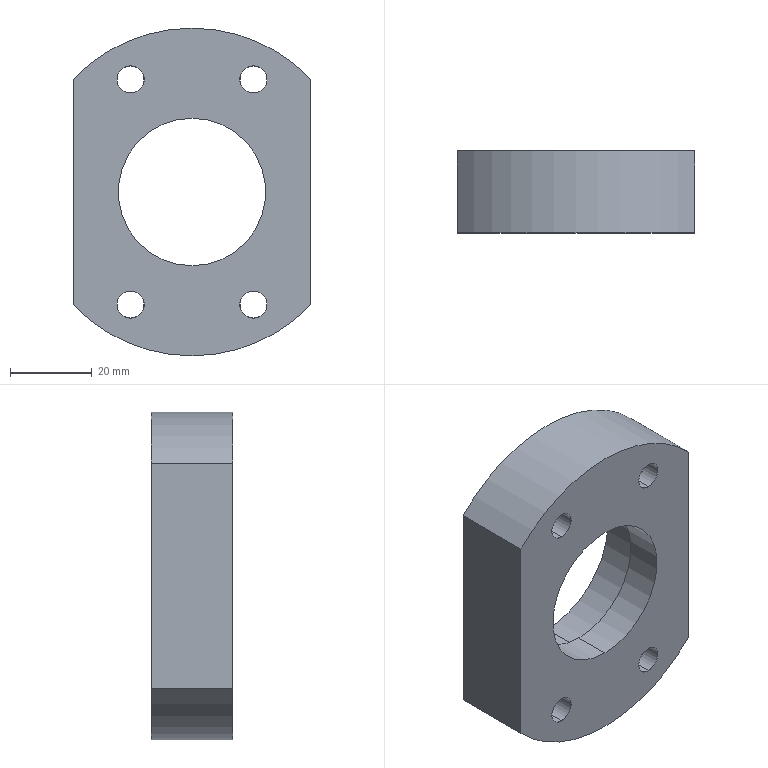Part | SolidWorks | features ICE 3, Extrusion 1, HoleWzd 1 | 1 solid | 28 faces | box 58 x 20 x 80 mm | volume 56726 mm3 | cylinder 15 | cone 8 | plane 5 | commonest cylinder face diameters 6.6 x8 80 x3 36 x2 42 x2
STEP:
#1=CARTESIAN_POINT('',(15.,0.025,30.8));
#2=VERTEX_POINT('',#1);
#3=CARTESIAN_POINT('',(15.,0.025,24.2));
#4=VERTEX_POINT('',#3);
#5=CARTESIAN_POINT('',(15.,0.025,27.5));
#6=DIRECTION('',(0.,-1.,0.));
#7=DIRECTION('',(0.,0.,-1.));
#8=AXIS2_PLACEMENT_3D('',#5,#6,#7);
#9=CIRCLE('',#8,3.3);
#10=EDGE_CURVE('',#2,#4,#9,.T.);
#11=ORIENTED_EDGE('',*,*,#10,.F.);
#12=CARTESIAN_POINT('',(15.,0.,30.825));
#13=VERTEX_POINT('',#12);
#14=CARTESIAN_POINT('',(15.,0.,30.825));
#15=DIRECTION('',(0.,-0.7071,0.7071));
#16=VECTOR('',#15,1000.);
#17=LINE('',#14,#16);
#18=EDGE_CURVE('',#2,#13,#17,.T.);
#19=ORIENTED_EDGE('',*,*,#18,.T.);
#20=CARTESIAN_POINT('',(15.,0.,24.175));
#21=VERTEX_POINT('',#20);
#22=CARTESIAN_POINT('',(15.,0.,27.5));
#23=DIRECTION('',(0.,-1.,0.));
#24=DIRECTION('',(0.,0.,-1.));
#25=AXIS2_PLACEMENT_3D('',#22,#23,#24);
#26=CIRCLE('',#25,3.325);
#27=EDGE_CURVE('',#13,#21,#26,.T.);
#28=ORIENTED_EDGE('',*,*,#27,.T.);
#29=CARTESIAN_POINT('',(15.,0.,24.175));
#30=DIRECTION('',(0.,-0.7071,-0.7071));
#31=VECTOR('',#30,1000.);
#32=LINE('',#29,#31);
#33=EDGE_CURVE('',#4,#21,#32,.T.);
#34=ORIENTED_EDGE('',*,*,#33,.F.);
#35=EDGE_LOOP('',(#11,#19,#28,#34));
#36=FACE_OUTER_BOUND('',#35,.T.);
#37=CARTESIAN_POINT('',(15.,0.,27.5));
#38=DIRECTION('',(0.,-1.,0.));
#39=DIRECTION('',(0.,0.,-1.));
#40=AXIS2_PLACEMENT_3D('',#37,#38,#39);
#41=CONICAL_SURFACE('',#40,3.325,0.7854);
#42=ADVANCED_FACE('',(#36),#41,.F.);
#43=CARTESIAN_POINT('',(15.,20.,30.8));
#44=VERTEX_POINT('',#43);
#45=CARTESIAN_POINT('',(15.,20.,24.2));
#46=VERTEX_POINT('',#45);
#47=CARTESIAN_POINT('',(15.,20.,27.5));
#48=DIRECTION('',(0.,-1.,0.));
#49=DIRECTION('',(0.,0.,-1.));
#50=AXIS2_PLACEMENT_3D('',#47,#48,#49);
#51=CIRCLE('',#50,3.3);
#52=EDGE_CURVE('',#44,#46,#51,.T.);
#53=ORIENTED_EDGE('',*,*,#52,.F.);
#54=CARTESIAN_POINT('',(15.,0.,30.8));
#55=DIRECTION('',(0.,-1.,0.));
#56=VECTOR('',#55,1000.);
#57=LINE('',#54,#56);
#58=EDGE_CURVE('',#44,#2,#57,.T.);
#59=ORIENTED_EDGE('',*,*,#58,.T.);
#60=ORIENTED_EDGE('',*,*,#10,.T.);
#61=CARTESIAN_POINT('',(15.,0.,24.2));
#62=DIRECTION('',(0.,-1.,0.));
#63=VECTOR('',#62,1000.);
#64=LINE('',#61,#63);
#65=EDGE_CURVE('',#46,#4,#64,.T.);
#66=ORIENTED_EDGE('',*,*,#65,.F.);
#67=EDGE_LOOP('',(#53,#59,#60,#66));
#68=FACE_OUTER_BOUND('',#67,.T.);
#69=CARTESIAN_POINT('',(15.,0.,27.5));
#70=DIRECTION('',(0.,-1.,0.));
#71=DIRECTION('',(0.,0.,-1.));
#72=AXIS2_PLACEMENT_3D('',#69,#70,#71);
#73=CYLINDRICAL_SURFACE('',#72,3.3);
#74=ADVANCED_FACE('',(#68),#73,.F.);
#75=CARTESIAN_POINT('',(-15.,0.025,30.8));
#76=VERTEX_POINT('',#75);
#77=CARTESIAN_POINT('',(-15.,0.025,24.2));
#78=VERTEX_POINT('',#77);
#79=CARTESIAN_POINT('',(-15.,0.025,27.5));
#80=DIRECTION('',(0.,-1.,0.));
#81=DIRECTION('',(0.,0.,-1.));
#82=AXIS2_PLACEMENT_3D('',#79,#80,#81);
#83=CIRCLE('',#82,3.3);
#84=EDGE_CURVE('',#76,#78,#83,.T.);
#85=ORIENTED_EDGE('',*,*,#84,.F.);
#86=CARTESIAN_POINT('',(-15.,0.,30.825));
#87=VERTEX_POINT('',#86);
#88=CARTESIAN_POINT('',(-15.,0.,30.825));
#89=DIRECTION('',(0.,-0.7071,0.7071));
#90=VECTOR('',#89,1000.);
#91=LINE('',#88,#90);
#92=EDGE_CURVE('',#76,#87,#91,.T.);
#93=ORIENTED_EDGE('',*,*,#92,.T.);
#94=CARTESIAN_POINT('',(-15.,0.,24.175));
#95=VERTEX_POINT('',#94);
#96=CARTESIAN_POINT('',(-15.,0.,27.5));
#97=DIRECTION('',(0.,-1.,0.));
#98=DIRECTION('',(0.,0.,-1.));
#99=AXIS2_PLACEMENT_3D('',#96,#97,#98);
#100=CIRCLE('',#99,3.325);
#101=EDGE_CURVE('',#87,#95,#100,.T.);
#102=ORIENTED_EDGE('',*,*,#101,.T.);
#103=CARTESIAN_POINT('',(-15.,0.,24.175));
#104=DIRECTION('',(0.,-0.7071,-0.7071));
#105=VECTOR('',#104,1000.);
#106=LINE('',#103,#105);
#107=EDGE_CURVE('',#78,#95,#106,.T.);
#108=ORIENTED_EDGE('',*,*,#107,.F.);
#109=EDGE_LOOP('',(#85,#93,#102,#108));
#110=FACE_OUTER_BOUND('',#109,.T.);
#111=CARTESIAN_POINT('',(-15.,0.,27.5));
#112=DIRECTION('',(0.,-1.,0.));
#113=DIRECTION('',(0.,0.,-1.));
#114=AXIS2_PLACEMENT_3D('',#111,#112,#113);
#115=CONICAL_SURFACE('',#114,3.325,0.7854);
#116=ADVANCED_FACE('',(#110),#115,.F.);
#117=CARTESIAN_POINT('',(-15.,20.,30.8));
#118=VERTEX_POINT('',#117);
#119=CARTESIAN_POINT('',(-15.,20.,24.2));
#120=VERTEX_POINT('',#119);
#121=CARTESIAN_POINT('',(-15.,20.,27.5));
#122=DIRECTION('',(0.,-1.,0.));
#123=DIRECTION('',(0.,0.,-1.));
#124=AXIS2_PLACEMENT_3D('',#121,#122,#123);
#125=CIRCLE('',#124,3.3);
#126=EDGE_CURVE('',#118,#120,#125,.T.);
#127=ORIENTED_EDGE('',*,*,#126,.F.);
#128=CARTESIAN_POINT('',(-15.,0.,30.8));
#129=DIRECTION('',(0.,-1.,0.));
#130=VECTOR('',#129,1000.);
#131=LINE('',#128,#130);
#132=EDGE_CURVE('',#118,#76,#131,.T.);
#133=ORIENTED_EDGE('',*,*,#132,.T.);
#134=ORIENTED_EDGE('',*,*,#84,.T.);
#135=CARTESIAN_POINT('',(-15.,0.,24.2));
#136=DIRECTION('',(0.,-1.,0.));
#137=VECTOR('',#136,1000.);
#138=LINE('',#135,#137);
#139=EDGE_CURVE('',#120,#78,#138,.T.);
#140=ORIENTED_EDGE('',*,*,#139,.F.);
#141=EDGE_LOOP('',(#127,#133,#134,#140));
#142=FACE_OUTER_BOUND('',#141,.T.);
#143=CARTESIAN_POINT('',(-15.,0.,27.5));
#144=DIRECTION('',(0.,-1.,0.));
#145=DIRECTION('',(0.,0.,-1.));
#146=AXIS2_PLACEMENT_3D('',#143,#144,#145);
#147=CYLINDRICAL_SURFACE('',#146,3.3);
#148=ADVANCED_FACE('',(#142),#147,.F.);
#149=CARTESIAN_POINT('',(-15.,0.025,-24.2));
#150=VERTEX_POINT('',#149);
#151=CARTESIAN_POINT('',(-15.,0.025,-30.8));
#152=VERTEX_POINT('',#151);
#153=CARTESIAN_POINT('',(-15.,0.025,-27.5));
#154=DIRECTION('',(0.,-1.,0.));
#155=DIRECTION('',(0.,0.,-1.));
#156=AXIS2_PLACEMENT_3D('',#153,#154,#155);
#157=CIRCLE('',#156,3.3);
#158=EDGE_CURVE('',#150,#152,#157,.T.);
#159=ORIENTED_EDGE('',*,*,#158,.F.);
#160=CARTESIAN_POINT('',(-15.,0.,-24.175));
#161=VERTEX_POINT('',#160);
#162=CARTESIAN_POINT('',(-15.,0.,-24.175));
#163=DIRECTION('',(0.,-0.7071,0.7071));
#164=VECTOR('',#163,1000.);
#165=LINE('',#162,#164);
#166=EDGE_CURVE('',#150,#161,#165,.T.);
#167=ORIENTED_EDGE('',*,*,#166,.T.);
#168=CARTESIAN_POINT('',(-15.,0.,-30.825));
#169=VERTEX_POINT('',#168);
#170=CARTESIAN_POINT('',(-15.,0.,-27.5));
#171=DIRECTION('',(0.,-1.,0.));
#172=DIRECTION('',(0.,0.,-1.));
#173=AXIS2_PLACEMENT_3D('',#170,#171,#172);
#174=CIRCLE('',#173,3.325);
#175=EDGE_CURVE('',#161,#169,#174,.T.);
#176=ORIENTED_EDGE('',*,*,#175,.T.);
#177=CARTESIAN_POINT('',(-15.,0.,-30.825));
#178=DIRECTION('',(0.,-0.7071,-0.7071));
#179=VECTOR('',#178,1000.);
#180=LINE('',#177,#179);
#181=EDGE_CURVE('',#152,#169,#180,.T.);
#182=ORIENTED_EDGE('',*,*,#181,.F.);
#183=EDGE_LOOP('',(#159,#167,#176,#182));
#184=FACE_OUTER_BOUND('',#183,.T.);
#185=CARTESIAN_POINT('',(-15.,0.,-27.5));
#186=DIRECTION('',(0.,-1.,0.));
#187=DIRECTION('',(0.,0.,-1.));
#188=AXIS2_PLACEMENT_3D('',#185,#186,#187);
#189=CONICAL_SURFACE('',#188,3.325,0.7854);
#190=ADVANCED_FACE('',(#184),#189,.F.);
#191=CARTESIAN_POINT('',(-15.,20.,-24.2));
#192=VERTEX_POINT('',#191);
#193=CARTESIAN_POINT('',(-15.,20.,-30.8));
#194=VERTEX_POINT('',#193);
#195=CARTESIAN_POINT('',(-15.,20.,-27.5));
#196=DIRECTION('',(0.,-1.,0.));
#197=DIRECTION('',(0.,0.,-1.));
#198=AXIS2_PLACEMENT_3D('',#195,#196,#197);
#199=CIRCLE('',#198,3.3);
#200=EDGE_CURVE('',#192,#194,#199,.T.);
#201=ORIENTED_EDGE('',*,*,#200,.F.);
#202=CARTESIAN_POINT('',(-15.,0.,-24.2));
#203=DIRECTION('',(0.,-1.,0.));
#204=VECTOR('',#203,1000.);
#205=LINE('',#202,#204);
#206=EDGE_CURVE('',#192,#150,#205,.T.);
#207=ORIENTED_EDGE('',*,*,#206,.T.);
#208=ORIENTED_EDGE('',*,*,#158,.T.);
#209=CARTESIAN_POINT('',(-15.,0.,-30.8));
#210=DIRECTION('',(0.,-1.,0.));
#211=VECTOR('',#210,1000.);
#212=LINE('',#209,#211);
#213=EDGE_CURVE('',#194,#152,#212,.T.);
#214=ORIENTED_EDGE('',*,*,#213,.F.);
#215=EDGE_LOOP('',(#201,#207,#208,#214));
#216=FACE_OUTER_BOUND('',#215,.T.);
#217=CARTESIAN_POINT('',(-15.,0.,-27.5));
#218=DIRECTION('',(0.,-1.,0.));
#219=DIRECTION('',(0.,0.,-1.));
#220=AXIS2_PLACEMENT_3D('',#217,#218,#219);
#221=CYLINDRICAL_SURFACE('',#220,3.3);
#222=ADVANCED_FACE('',(#216),#221,.F.);
#223=CARTESIAN_POINT('',(15.,0.025,-24.2));
#224=VERTEX_POINT('',#223);
#225=CARTESIAN_POINT('',(15.,0.025,-30.8));
#226=VERTEX_POINT('',#225);
#227=CARTESIAN_POINT('',(15.,0.025,-27.5));
#228=DIRECTION('',(0.,-1.,0.));
#229=DIRECTION('',(0.,0.,-1.));
#230=AXIS2_PLACEMENT_3D('',#227,#228,#229);
#231=CIRCLE('',#230,3.3);
#232=EDGE_CURVE('',#224,#226,#231,.T.);
#233=ORIENTED_EDGE('',*,*,#232,.F.);
#234=CARTESIAN_POINT('',(15.,0.,-24.175));
#235=VERTEX_POINT('',#234);
#236=CARTESIAN_POINT('',(15.,0.,-24.175));
#237=DIRECTION('',(0.,-0.7071,0.7071));
#238=VECTOR('',#237,1000.);
#239=LINE('',#236,#238);
#240=EDGE_CURVE('',#224,#235,#239,.T.);
#241=ORIENTED_EDGE('',*,*,#240,.T.);
#242=CARTESIAN_POINT('',(15.,0.,-30.825));
#243=VERTEX_POINT('',#242);
#244=CARTESIAN_POINT('',(15.,0.,-27.5));
#245=DIRECTION('',(0.,-1.,0.));
#246=DIRECTION('',(0.,0.,-1.));
#247=AXIS2_PLACEMENT_3D('',#244,#245,#246);
#248=CIRCLE('',#247,3.325);
#249=EDGE_CURVE('',#235,#243,#248,.T.);
#250=ORIENTED_EDGE('',*,*,#249,.T.);
#251=CARTESIAN_POINT('',(15.,0.,-30.825));
#252=DIRECTION('',(0.,-0.7071,-0.7071));
#253=VECTOR('',#252,1000.);
#254=LINE('',#251,#253);
#255=EDGE_CURVE('',#226,#243,#254,.T.);
#256=ORIENTED_EDGE('',*,*,#255,.F.);
#257=EDGE_LOOP('',(#233,#241,#250,#256));
#258=FACE_OUTER_BOUND('',#257,.T.);
#259=CARTESIAN_POINT('',(15.,0.,-27.5));
#260=DIRECTION('',(0.,-1.,0.));
#261=DIRECTION('',(0.,0.,-1.));
#262=AXIS2_PLACEMENT_3D('',#259,#260,#261);
#263=CONICAL_SURFACE('',#262,3.325,0.7854);
#264=ADVANCED_FACE('',(#258),#263,.F.);
#265=CARTESIAN_POINT('',(15.,20.,-24.2));
#266=VERTEX_POINT('',#265);
#267=CARTESIAN_POINT('',(15.,20.,-30.8));
#268=VERTEX_POINT('',#267);
#269=CARTESIAN_POINT('',(15.,20.,-27.5));
#270=DIRECTION('',(0.,-1.,0.));
#271=DIRECTION('',(0.,0.,-1.));
#272=AXIS2_PLACEMENT_3D('',#269,#270,#271);
#273=CIRCLE('',#272,3.3);
#274=EDGE_CURVE('',#266,#268,#273,.T.);
#275=ORIENTED_EDGE('',*,*,#274,.F.);
#276=CARTESIAN_POINT('',(15.,0.,-24.2));
#277=DIRECTION('',(0.,-1.,0.));
#278=VECTOR('',#277,1000.);
#279=LINE('',#276,#278);
#280=EDGE_CURVE('',#266,#224,#279,.T.);
#281=ORIENTED_EDGE('',*,*,#280,.T.);
#282=ORIENTED_EDGE('',*,*,#232,.T.);
#283=CARTESIAN_POINT('',(15.,0.,-30.8));
#284=DIRECTION('',(0.,-1.,0.));
#285=VECTOR('',#284,1000.);
#286=LINE('',#283,#285);
#287=EDGE_CURVE('',#268,#226,#286,.T.);
#288=ORIENTED_EDGE('',*,*,#287,.F.);
#289=EDGE_LOOP('',(#275,#281,#282,#288));
#290=FACE_OUTER_BOUND('',#289,.T.);
#291=CARTESIAN_POINT('',(15.,0.,-27.5));
#292=DIRECTION('',(0.,-1.,0.));
#293=DIRECTION('',(0.,0.,-1.));
#294=AXIS2_PLACEMENT_3D('',#291,#292,#293);
#295=CYLINDRICAL_SURFACE('',#294,3.3);
#296=ADVANCED_FACE('',(#290),#295,.F.);
#297=CARTESIAN_POINT('',(0.,0.,-18.));
#298=VERTEX_POINT('',#297);
#299=CARTESIAN_POINT('',(0.,0.,18.));
#300=VERTEX_POINT('',#299);
#301=CARTESIAN_POINT('',(0.,0.,0.));
#302=DIRECTION('',(0.,1.,0.));
#303=DIRECTION('',(0.,0.,1.));
#304=AXIS2_PLACEMENT_3D('',#301,#302,#303);
#305=CIRCLE('',#304,18.);
#306=EDGE_CURVE('',#298,#300,#305,.T.);
#307=ORIENTED_EDGE('',*,*,#306,.F.);
#308=CARTESIAN_POINT('',(0.,9.,-18.));
#309=VERTEX_POINT('',#308);
#310=CARTESIAN_POINT('',(0.,-2.,-18.));
#311=DIRECTION('',(0.,1.,0.));
#312=VECTOR('',#311,1000.);
#313=LINE('',#310,#312);
#314=EDGE_CURVE('',#298,#309,#313,.T.);
#315=ORIENTED_EDGE('',*,*,#314,.T.);
#316=CARTESIAN_POINT('',(0.,9.,18.));
#317=VERTEX_POINT('',#316);
#318=CARTESIAN_POINT('',(0.,9.,0.));
#319=DIRECTION('',(0.,1.,0.));
#320=DIRECTION('',(0.,0.,1.));
#321=AXIS2_PLACEMENT_3D('',#318,#319,#320);
#322=CIRCLE('',#321,18.);
#323=EDGE_CURVE('',#309,#317,#322,.T.);
#324=ORIENTED_EDGE('',*,*,#323,.T.);
#325=CARTESIAN_POINT('',(0.,-2.,18.));
#326=DIRECTION('',(0.,1.,0.));
#327=VECTOR('',#326,1000.);
#328=LINE('',#325,#327);
#329=EDGE_CURVE('',#300,#317,#328,.T.);
#330=ORIENTED_EDGE('',*,*,#329,.F.);
#331=EDGE_LOOP('',(#307,#315,#324,#330));
#332=FACE_OUTER_BOUND('',#331,.T.);
#333=CARTESIAN_POINT('',(0.,-2.,0.));
#334=DIRECTION('',(0.,1.,0.));
#335=DIRECTION('',(0.,0.,1.));
#336=AXIS2_PLACEMENT_3D('',#333,#334,#335);
#337=CYLINDRICAL_SURFACE('',#336,18.);
#338=ADVANCED_FACE('',(#332),#337,.F.);
#339=CARTESIAN_POINT('',(0.,9.,-21.));
#340=VERTEX_POINT('',#339);
#341=CARTESIAN_POINT('',(0.,9.,21.));
#342=VERTEX_POINT('',#341);
#343=CARTESIAN_POINT('',(0.,9.,0.));
#344=DIRECTION('',(0.,1.,0.));
#345=DIRECTION('',(0.,0.,1.));
#346=AXIS2_PLACEMENT_3D('',#343,#344,#345);
#347=CIRCLE('',#346,21.);
#348=EDGE_CURVE('',#340,#342,#347,.T.);
#349=ORIENTED_EDGE('',*,*,#348,.F.);
#350=CARTESIAN_POINT('',(0.,20.,-21.));
#351=VERTEX_POINT('',#350);
#352=CARTESIAN_POINT('',(0.,9.,-21.));
#353=DIRECTION('',(0.,1.,0.));
#354=VECTOR('',#353,1000.);
#355=LINE('',#352,#354);
#356=EDGE_CURVE('',#340,#351,#355,.T.);
#357=ORIENTED_EDGE('',*,*,#356,.T.);
#358=CARTESIAN_POINT('',(0.,20.,21.));
#359=VERTEX_POINT('',#358);
#360=CARTESIAN_POINT('',(0.,20.,0.));
#361=DIRECTION('',(0.,1.,0.));
#362=DIRECTION('',(0.,0.,1.));
#363=AXIS2_PLACEMENT_3D('',#360,#361,#362);
#364=CIRCLE('',#363,21.);
#365=EDGE_CURVE('',#351,#359,#364,.T.);
#366=ORIENTED_EDGE('',*,*,#365,.T.);
#367=CARTESIAN_POINT('',(0.,9.,21.));
#368=DIRECTION('',(0.,1.,0.));
#369=VECTOR('',#368,1000.);
#370=LINE('',#367,#369);
#371=EDGE_CURVE('',#342,#359,#370,.T.);
#372=ORIENTED_EDGE('',*,*,#371,.F.);
#373=EDGE_LOOP('',(#349,#357,#366,#372));
#374=FACE_OUTER_BOUND('',#373,.T.);
#375=CARTESIAN_POINT('',(0.,9.,0.));
#376=DIRECTION('',(0.,1.,0.));
#377=DIRECTION('',(0.,0.,1.));
#378=AXIS2_PLACEMENT_3D('',#375,#376,#377);
#379=CYLINDRICAL_SURFACE('',#378,21.);
#380=ADVANCED_FACE('',(#374),#379,.F.);
#381=CARTESIAN_POINT('',(0.,20.,-40.));
#382=VERTEX_POINT('',#381);
#383=CARTESIAN_POINT('',(-29.,20.,-27.55));
#384=VERTEX_POINT('',#383);
#385=CARTESIAN_POINT('',(0.,20.,0.));
#386=DIRECTION('',(0.,1.,0.));
#387=DIRECTION('',(0.,0.,1.));
#388=AXIS2_PLACEMENT_3D('',#385,#386,#387);
#389=CIRCLE('',#388,40.);
#390=EDGE_CURVE('',#382,#384,#389,.T.);
#391=ORIENTED_EDGE('',*,*,#390,.F.);
#392=CARTESIAN_POINT('',(0.,0.,-40.));
#393=VERTEX_POINT('',#392);
#394=CARTESIAN_POINT('',(0.,20.,-40.));
#395=DIRECTION('',(0.,-1.,0.));
#396=VECTOR('',#395,1000.);
#397=LINE('',#394,#396);
#398=EDGE_CURVE('',#382,#393,#397,.T.);
#399=ORIENTED_EDGE('',*,*,#398,.T.);
#400=CARTESIAN_POINT('',(-29.,0.,-27.55));
#401=VERTEX_POINT('',#400);
#402=CARTESIAN_POINT('',(0.,0.,0.));
#403=DIRECTION('',(0.,1.,0.));
#404=DIRECTION('',(0.,0.,1.));
#405=AXIS2_PLACEMENT_3D('',#402,#403,#404);
#406=CIRCLE('',#405,40.);
#407=EDGE_CURVE('',#393,#401,#406,.T.);
#408=ORIENTED_EDGE('',*,*,#407,.T.);
#409=CARTESIAN_POINT('',(-29.,20.,-27.55));
#410=DIRECTION('',(0.,-1.,0.));
#411=VECTOR('',#410,1000.);
#412=LINE('',#409,#411);
#413=EDGE_CURVE('',#384,#401,#412,.T.);
#414=ORIENTED_EDGE('',*,*,#413,.F.);
#415=EDGE_LOOP('',(#391,#399,#408,#414));
#416=FACE_OUTER_BOUND('',#415,.T.);
#417=CARTESIAN_POINT('',(0.,20.,0.));
#418=DIRECTION('',(0.,-1.,0.));
#419=DIRECTION('',(0.,0.,-1.));
#420=AXIS2_PLACEMENT_3D('',#417,#418,#419);
#421=CYLINDRICAL_SURFACE('',#420,40.);
#422=ADVANCED_FACE('',(#416),#421,.T.);
#423=CARTESIAN_POINT('',(29.,20.,27.55));
#424=VERTEX_POINT('',#423);
#425=CARTESIAN_POINT('',(29.,0.,27.55));
#426=VERTEX_POINT('',#425);
#427=CARTESIAN_POINT('',(29.,20.,27.55));
#428=DIRECTION('',(0.,-1.,0.));
#429=VECTOR('',#428,1000.);
#430=LINE('',#427,#429);
#431=EDGE_CURVE('',#424,#426,#430,.T.);
#432=ORIENTED_EDGE('',*,*,#431,.F.);
#433=CARTESIAN_POINT('',(-29.,20.,27.55));
#434=VERTEX_POINT('',#433);
#435=CARTESIAN_POINT('',(0.,20.,0.));
#436=DIRECTION('',(0.,1.,0.));
#437=DIRECTION('',(0.,0.,1.));
#438=AXIS2_PLACEMENT_3D('',#435,#436,#437);
#439=CIRCLE('',#438,40.);
#440=EDGE_CURVE('',#434,#424,#439,.T.);
#441=ORIENTED_EDGE('',*,*,#440,.F.);
#442=CARTESIAN_POINT('',(-29.,0.,27.55));
#443=VERTEX_POINT('',#442);
#444=CARTESIAN_POINT('',(-29.,20.,27.55));
#445=DIRECTION('',(0.,-1.,0.));
#446=VECTOR('',#445,1000.);
#447=LINE('',#444,#446);
#448=EDGE_CURVE('',#434,#443,#447,.T.);
#449=ORIENTED_EDGE('',*,*,#448,.T.);
#450=CARTESIAN_POINT('',(0.,0.,0.));
#451=DIRECTION('',(0.,1.,0.));
#452=DIRECTION('',(0.,0.,1.));
#453=AXIS2_PLACEMENT_3D('',#450,#451,#452);
#454=CIRCLE('',#453,40.);
#455=EDGE_CURVE('',#443,#426,#454,.T.);
#456=ORIENTED_EDGE('',*,*,#455,.T.);
#457=EDGE_LOOP('',(#432,#441,#449,#456));
#458=FACE_OUTER_BOUND('',#457,.T.);
#459=CARTESIAN_POINT('',(0.,20.,0.));
#460=DIRECTION('',(0.,-1.,0.));
#461=DIRECTION('',(0.,0.,-1.));
#462=AXIS2_PLACEMENT_3D('',#459,#460,#461);
#463=CYLINDRICAL_SURFACE('',#462,40.);
#464=ADVANCED_FACE('',(#458),#463,.T.);
#465=ORIENTED_EDGE('',*,*,#398,.F.);
#466=CARTESIAN_POINT('',(29.,20.,-27.55));
#467=VERTEX_POINT('',#466);
#468=CARTESIAN_POINT('',(0.,20.,0.));
#469=DIRECTION('',(0.,1.,0.));
#470=DIRECTION('',(0.,0.,1.));
#471=AXIS2_PLACEMENT_3D('',#468,#469,#470);
#472=CIRCLE('',#471,40.);
#473=EDGE_CURVE('',#467,#382,#472,.T.);
#474=ORIENTED_EDGE('',*,*,#473,.F.);
#475=CARTESIAN_POINT('',(29.,0.,-27.55));
#476=VERTEX_POINT('',#475);
#477=CARTESIAN_POINT('',(29.,20.,-27.55));
#478=DIRECTION('',(0.,-1.,0.));
#479=VECTOR('',#478,1000.);
#480=LINE('',#477,#479);
#481=EDGE_CURVE('',#467,#476,#480,.T.);
#482=ORIENTED_EDGE('',*,*,#481,.T.);
#483=CARTESIAN_POINT('',(0.,0.,0.));
#484=DIRECTION('',(0.,1.,0.));
#485=DIRECTION('',(0.,0.,1.));
#486=AXIS2_PLACEMENT_3D('',#483,#484,#485);
#487=CIRCLE('',#486,40.);
#488=EDGE_CURVE('',#476,#393,#487,.T.);
#489=ORIENTED_EDGE('',*,*,#488,.T.);
#490=EDGE_LOOP('',(#465,#474,#482,#489));
#491=FACE_OUTER_BOUND('',#490,.T.);
#492=CARTESIAN_POINT('',(0.,20.,0.));
#493=DIRECTION('',(0.,-1.,0.));
#494=DIRECTION('',(0.,0.,-1.));
#495=AXIS2_PLACEMENT_3D('',#492,#493,#494);
#496=CYLINDRICAL_SURFACE('',#495,40.);
#497=ADVANCED_FACE('',(#491),#496,.T.);
#498=CARTESIAN_POINT('',(15.,20.,27.5));
#499=DIRECTION('',(0.,-1.,0.));
#500=DIRECTION('',(0.,0.,-1.));
#501=AXIS2_PLACEMENT_3D('',#498,#499,#500);
#502=CIRCLE('',#501,3.3);
#503=EDGE_CURVE('',#46,#44,#502,.T.);
#504=ORIENTED_EDGE('',*,*,#503,.T.);
#505=ORIENTED_EDGE('',*,*,#52,.T.);
#506=EDGE_LOOP('',(#504,#505));
#507=FACE_BOUND('',#506,.T.);
#508=CARTESIAN_POINT('',(-15.,20.,27.5));
#509=DIRECTION('',(0.,-1.,0.));
#510=DIRECTION('',(0.,0.,-1.));
#511=AXIS2_PLACEMENT_3D('',#508,#509,#510);
#512=CIRCLE('',#511,3.3);
#513=EDGE_CURVE('',#120,#118,#512,.T.);
#514=ORIENTED_EDGE('',*,*,#513,.T.);
#515=ORIENTED_EDGE('',*,*,#126,.T.);
#516=EDGE_LOOP('',(#514,#515));
#517=FACE_BOUND('',#516,.T.);
#518=CARTESIAN_POINT('',(-15.,20.,-27.5));
#519=DIRECTION('',(0.,-1.,0.));
#520=DIRECTION('',(0.,0.,-1.));
#521=AXIS2_PLACEMENT_3D('',#518,#519,#520);
#522=CIRCLE('',#521,3.3);
#523=EDGE_CURVE('',#194,#192,#522,.T.);
#524=ORIENTED_EDGE('',*,*,#523,.T.);
#525=ORIENTED_EDGE('',*,*,#200,.T.);
#526=EDGE_LOOP('',(#524,#525));
#527=FACE_BOUND('',#526,.T.);
#528=CARTESIAN_POINT('',(15.,20.,-27.5));
#529=DIRECTION('',(0.,-1.,0.));
#530=DIRECTION('',(0.,0.,-1.));
#531=AXIS2_PLACEMENT_3D('',#528,#529,#530);
#532=CIRCLE('',#531,3.3);
#533=EDGE_CURVE('',#268,#266,#532,.T.);
#534=ORIENTED_EDGE('',*,*,#533,.T.);
#535=ORIENTED_EDGE('',*,*,#274,.T.);
#536=EDGE_LOOP('',(#534,#535));
#537=FACE_BOUND('',#536,.T.);
#538=CARTESIAN_POINT('',(0.,20.,0.));
#539=DIRECTION('',(0.,1.,0.));
#540=DIRECTION('',(0.,0.,1.));
#541=AXIS2_PLACEMENT_3D('',#538,#539,#540);
#542=CIRCLE('',#541,21.);
#543=EDGE_CURVE('',#359,#351,#542,.T.);
#544=ORIENTED_EDGE('',*,*,#543,.F.);
#545=ORIENTED_EDGE('',*,*,#365,.F.);
#546=EDGE_LOOP('',(#544,#545));
#547=FACE_BOUND('',#546,.T.);
#548=ORIENTED_EDGE('',*,*,#440,.T.);
#549=CARTESIAN_POINT('',(29.,20.,0.));
#550=DIRECTION('',(0.,0.,1.));
#551=VECTOR('',#550,1000.);
#552=LINE('',#549,#551);
#553=EDGE_CURVE('',#467,#424,#552,.T.);
#554=ORIENTED_EDGE('',*,*,#553,.F.);
#555=ORIENTED_EDGE('',*,*,#473,.T.);
#556=ORIENTED_EDGE('',*,*,#390,.T.);
#557=CARTESIAN_POINT('',(-29.,20.,0.));
#558=DIRECTION('',(0.,0.,1.));
#559=VECTOR('',#558,1000.);
#560=LINE('',#557,#559);
#561=EDGE_CURVE('',#384,#434,#560,.T.);
#562=ORIENTED_EDGE('',*,*,#561,.T.);
#563=EDGE_LOOP('',(#548,#554,#555,#556,#562));
#564=FACE_OUTER_BOUND('',#563,.T.);
#565=CARTESIAN_POINT('',(0.,20.,0.));
#566=DIRECTION('',(0.,1.,0.));
#567=DIRECTION('',(0.,0.,1.));
#568=AXIS2_PLACEMENT_3D('',#565,#566,#567);
#569=PLANE('',#568);
#570=ADVANCED_FACE('',(#507,#517,#527,#537,#547,#564),#569,.T.);
#571=CARTESIAN_POINT('',(15.,0.,27.5));
#572=DIRECTION('',(0.,-1.,0.));
#573=DIRECTION('',(0.,0.,-1.));
#574=AXIS2_PLACEMENT_3D('',#571,#572,#573);
#575=CIRCLE('',#574,3.325);
#576=EDGE_CURVE('',#21,#13,#575,.T.);
#577=ORIENTED_EDGE('',*,*,#576,.F.);
#578=ORIENTED_EDGE('',*,*,#27,.F.);
#579=EDGE_LOOP('',(#577,#578));
#580=FACE_BOUND('',#579,.T.);
#581=CARTESIAN_POINT('',(-15.,0.,27.5));
#582=DIRECTION('',(0.,-1.,0.));
#583=DIRECTION('',(0.,0.,-1.));
#584=AXIS2_PLACEMENT_3D('',#581,#582,#583);
#585=CIRCLE('',#584,3.325);
#586=EDGE_CURVE('',#95,#87,#585,.T.);
#587=ORIENTED_EDGE('',*,*,#586,.F.);
#588=ORIENTED_EDGE('',*,*,#101,.F.);
#589=EDGE_LOOP('',(#587,#588));
#590=FACE_BOUND('',#589,.T.);
#591=CARTESIAN_POINT('',(-15.,0.,-27.5));
#592=DIRECTION('',(0.,-1.,0.));
#593=DIRECTION('',(0.,0.,-1.));
#594=AXIS2_PLACEMENT_3D('',#591,#592,#593);
#595=CIRCLE('',#594,3.325);
#596=EDGE_CURVE('',#169,#161,#595,.T.);
#597=ORIENTED_EDGE('',*,*,#596,.F.);
#598=ORIENTED_EDGE('',*,*,#175,.F.);
#599=EDGE_LOOP('',(#597,#598));
#600=FACE_BOUND('',#599,.T.);
#601=CARTESIAN_POINT('',(15.,0.,-27.5));
#602=DIRECTION('',(0.,-1.,0.));
#603=DIRECTION('',(0.,0.,-1.));
#604=AXIS2_PLACEMENT_3D('',#601,#602,#603);
#605=CIRCLE('',#604,3.325);
#606=EDGE_CURVE('',#243,#235,#605,.T.);
#607=ORIENTED_EDGE('',*,*,#606,.F.);
#608=ORIENTED_EDGE('',*,*,#249,.F.);
#609=EDGE_LOOP('',(#607,#608));
#610=FACE_BOUND('',#609,.T.);
#611=CARTESIAN_POINT('',(0.,0.,0.));
#612=DIRECTION('',(0.,1.,0.));
#613=DIRECTION('',(0.,0.,1.));
#614=AXIS2_PLACEMENT_3D('',#611,#612,#613);
#615=CIRCLE('',#614,18.);
#616=EDGE_CURVE('',#300,#298,#615,.T.);
#617=ORIENTED_EDGE('',*,*,#616,.T.);
#618=ORIENTED_EDGE('',*,*,#306,.T.);
#619=EDGE_LOOP('',(#617,#618));
#620=FACE_BOUND('',#619,.T.);
#621=CARTESIAN_POINT('',(29.,0.,0.));
#622=DIRECTION('',(0.,0.,1.));
#623=VECTOR('',#622,1000.);
#624=LINE('',#621,#623);
#625=EDGE_CURVE('',#476,#426,#624,.T.);
#626=ORIENTED_EDGE('',*,*,#625,.T.);
#627=ORIENTED_EDGE('',*,*,#455,.F.);
#628=CARTESIAN_POINT('',(-29.,0.,0.));
#629=DIRECTION('',(0.,0.,1.));
#630=VECTOR('',#629,1000.);
#631=LINE('',#628,#630);
#632=EDGE_CURVE('',#401,#443,#631,.T.);
#633=ORIENTED_EDGE('',*,*,#632,.F.);
#634=ORIENTED_EDGE('',*,*,#407,.F.);
#635=ORIENTED_EDGE('',*,*,#488,.F.);
#636=EDGE_LOOP('',(#626,#627,#633,#634,#635));
#637=FACE_OUTER_BOUND('',#636,.T.);
#638=CARTESIAN_POINT('',(0.,0.,0.));
#639=DIRECTION('',(0.,1.,0.));
#640=DIRECTION('',(0.,0.,1.));
#641=AXIS2_PLACEMENT_3D('',#638,#639,#640);
#642=PLANE('',#641);
#643=ADVANCED_FACE('',(#580,#590,#600,#610,#620,#637),#642,.F.);
#644=ORIENTED_EDGE('',*,*,#356,.F.);
#645=CARTESIAN_POINT('',(0.,9.,0.));
#646=DIRECTION('',(0.,1.,0.));
#647=DIRECTION('',(0.,0.,1.));
#648=AXIS2_PLACEMENT_3D('',#645,#646,#647);
#649=CIRCLE('',#648,21.);
#650=EDGE_CURVE('',#342,#340,#649,.T.);
#651=ORIENTED_EDGE('',*,*,#650,.F.);
#652=ORIENTED_EDGE('',*,*,#371,.T.);
#653=ORIENTED_EDGE('',*,*,#543,.T.);
#654=EDGE_LOOP('',(#644,#651,#652,#653));
#655=FACE_OUTER_BOUND('',#654,.T.);
#656=CARTESIAN_POINT('',(0.,9.,0.));
#657=DIRECTION('',(0.,1.,0.));
#658=DIRECTION('',(0.,0.,1.));
#659=AXIS2_PLACEMENT_3D('',#656,#657,#658);
#660=CYLINDRICAL_SURFACE('',#659,21.);
#661=ADVANCED_FACE('',(#655),#660,.F.);
#662=CARTESIAN_POINT('',(0.,9.,0.));
#663=DIRECTION('',(0.,1.,0.));
#664=DIRECTION('',(0.,0.,1.));
#665=AXIS2_PLACEMENT_3D('',#662,#663,#664);
#666=CIRCLE('',#665,18.);
#667=EDGE_CURVE('',#317,#309,#666,.T.);
#668=ORIENTED_EDGE('',*,*,#667,.F.);
#669=ORIENTED_EDGE('',*,*,#323,.F.);
#670=EDGE_LOOP('',(#668,#669));
#671=FACE_BOUND('',#670,.T.);
#672=ORIENTED_EDGE('',*,*,#650,.T.);
#673=ORIENTED_EDGE('',*,*,#348,.T.);
#674=EDGE_LOOP('',(#672,#673));
#675=FACE_OUTER_BOUND('',#674,.T.);
#676=CARTESIAN_POINT('',(0.,9.,0.));
#677=DIRECTION('',(0.,1.,0.));
#678=DIRECTION('',(0.,0.,1.));
#679=AXIS2_PLACEMENT_3D('',#676,#677,#678);
#680=PLANE('',#679);
#681=ADVANCED_FACE('',(#671,#675),#680,.T.);
#682=ORIENTED_EDGE('',*,*,#314,.F.);
#683=ORIENTED_EDGE('',*,*,#616,.F.);
#684=ORIENTED_EDGE('',*,*,#329,.T.);
#685=ORIENTED_EDGE('',*,*,#667,.T.);
#686=EDGE_LOOP('',(#682,#683,#684,#685));
#687=FACE_OUTER_BOUND('',#686,.T.);
#688=CARTESIAN_POINT('',(0.,-2.,0.));
#689=DIRECTION('',(0.,1.,0.));
#690=DIRECTION('',(0.,0.,1.));
#691=AXIS2_PLACEMENT_3D('',#688,#689,#690);
#692=CYLINDRICAL_SURFACE('',#691,18.);
#693=ADVANCED_FACE('',(#687),#692,.F.);
#694=ORIENTED_EDGE('',*,*,#632,.T.);
#695=ORIENTED_EDGE('',*,*,#448,.F.);
#696=ORIENTED_EDGE('',*,*,#561,.F.);
#697=ORIENTED_EDGE('',*,*,#413,.T.);
#698=EDGE_LOOP('',(#694,#695,#696,#697));
#699=FACE_OUTER_BOUND('',#698,.T.);
#700=CARTESIAN_POINT('',(-29.,20.,0.));
#701=DIRECTION('',(1.,0.,0.));
#702=DIRECTION('',(0.,0.,-1.));
#703=AXIS2_PLACEMENT_3D('',#700,#701,#702);
#704=PLANE('',#703);
#705=ADVANCED_FACE('',(#699),#704,.F.);
#706=ORIENTED_EDGE('',*,*,#625,.F.);
#707=ORIENTED_EDGE('',*,*,#481,.F.);
#708=ORIENTED_EDGE('',*,*,#553,.T.);
#709=ORIENTED_EDGE('',*,*,#431,.T.);
#710=EDGE_LOOP('',(#706,#707,#708,#709));
#711=FACE_OUTER_BOUND('',#710,.T.);
#712=CARTESIAN_POINT('',(29.,20.,0.));
#713=DIRECTION('',(1.,0.,0.));
#714=DIRECTION('',(0.,0.,-1.));
#715=AXIS2_PLACEMENT_3D('',#712,#713,#714);
#716=PLANE('',#715);
#717=ADVANCED_FACE('',(#711),#716,.T.);
#718=ORIENTED_EDGE('',*,*,#280,.F.);
#719=ORIENTED_EDGE('',*,*,#533,.F.);
#720=ORIENTED_EDGE('',*,*,#287,.T.);
#721=CARTESIAN_POINT('',(15.,0.025,-27.5));
#722=DIRECTION('',(0.,-1.,0.));
#723=DIRECTION('',(0.,0.,-1.));
#724=AXIS2_PLACEMENT_3D('',#721,#722,#723);
#725=CIRCLE('',#724,3.3);
#726=EDGE_CURVE('',#226,#224,#725,.T.);
#727=ORIENTED_EDGE('',*,*,#726,.T.);
#728=EDGE_LOOP('',(#718,#719,#720,#727));
#729=FACE_OUTER_BOUND('',#728,.T.);
#730=CARTESIAN_POINT('',(15.,0.,-27.5));
#731=DIRECTION('',(0.,-1.,0.));
#732=DIRECTION('',(0.,0.,-1.));
#733=AXIS2_PLACEMENT_3D('',#730,#731,#732);
#734=CYLINDRICAL_SURFACE('',#733,3.3);
#735=ADVANCED_FACE('',(#729),#734,.F.);
#736=ORIENTED_EDGE('',*,*,#240,.F.);
#737=ORIENTED_EDGE('',*,*,#726,.F.);
#738=ORIENTED_EDGE('',*,*,#255,.T.);
#739=ORIENTED_EDGE('',*,*,#606,.T.);
#740=EDGE_LOOP('',(#736,#737,#738,#739));
#741=FACE_OUTER_BOUND('',#740,.T.);
#742=CARTESIAN_POINT('',(15.,0.,-27.5));
#743=DIRECTION('',(0.,-1.,0.));
#744=DIRECTION('',(0.,0.,-1.));
#745=AXIS2_PLACEMENT_3D('',#742,#743,#744);
#746=CONICAL_SURFACE('',#745,3.325,0.7854);
#747=ADVANCED_FACE('',(#741),#746,.F.);
#748=ORIENTED_EDGE('',*,*,#206,.F.);
#749=ORIENTED_EDGE('',*,*,#523,.F.);
#750=ORIENTED_EDGE('',*,*,#213,.T.);
#751=CARTESIAN_POINT('',(-15.,0.025,-27.5));
#752=DIRECTION('',(0.,-1.,0.));
#753=DIRECTION('',(0.,0.,-1.));
#754=AXIS2_PLACEMENT_3D('',#751,#752,#753);
#755=CIRCLE('',#754,3.3);
#756=EDGE_CURVE('',#152,#150,#755,.T.);
#757=ORIENTED_EDGE('',*,*,#756,.T.);
#758=EDGE_LOOP('',(#748,#749,#750,#757));
#759=FACE_OUTER_BOUND('',#758,.T.);
#760=CARTESIAN_POINT('',(-15.,0.,-27.5));
#761=DIRECTION('',(0.,-1.,0.));
#762=DIRECTION('',(0.,0.,-1.));
#763=AXIS2_PLACEMENT_3D('',#760,#761,#762);
#764=CYLINDRICAL_SURFACE('',#763,3.3);
#765=ADVANCED_FACE('',(#759),#764,.F.);
#766=ORIENTED_EDGE('',*,*,#166,.F.);
#767=ORIENTED_EDGE('',*,*,#756,.F.);
#768=ORIENTED_EDGE('',*,*,#181,.T.);
#769=ORIENTED_EDGE('',*,*,#596,.T.);
#770=EDGE_LOOP('',(#766,#767,#768,#769));
#771=FACE_OUTER_BOUND('',#770,.T.);
#772=CARTESIAN_POINT('',(-15.,0.,-27.5));
#773=DIRECTION('',(0.,-1.,0.));
#774=DIRECTION('',(0.,0.,-1.));
#775=AXIS2_PLACEMENT_3D('',#772,#773,#774);
#776=CONICAL_SURFACE('',#775,3.325,0.7854);
#777=ADVANCED_FACE('',(#771),#776,.F.);
#778=ORIENTED_EDGE('',*,*,#132,.F.);
#779=ORIENTED_EDGE('',*,*,#513,.F.);
#780=ORIENTED_EDGE('',*,*,#139,.T.);
#781=CARTESIAN_POINT('',(-15.,0.025,27.5));
#782=DIRECTION('',(0.,-1.,0.));
#783=DIRECTION('',(0.,0.,-1.));
#784=AXIS2_PLACEMENT_3D('',#781,#782,#783);
#785=CIRCLE('',#784,3.3);
#786=EDGE_CURVE('',#78,#76,#785,.T.);
#787=ORIENTED_EDGE('',*,*,#786,.T.);
#788=EDGE_LOOP('',(#778,#779,#780,#787));
#789=FACE_OUTER_BOUND('',#788,.T.);
#790=CARTESIAN_POINT('',(-15.,0.,27.5));
#791=DIRECTION('',(0.,-1.,0.));
#792=DIRECTION('',(0.,0.,-1.));
#793=AXIS2_PLACEMENT_3D('',#790,#791,#792);
#794=CYLINDRICAL_SURFACE('',#793,3.3);
#795=ADVANCED_FACE('',(#789),#794,.F.);
#796=ORIENTED_EDGE('',*,*,#92,.F.);
#797=ORIENTED_EDGE('',*,*,#786,.F.);
#798=ORIENTED_EDGE('',*,*,#107,.T.);
#799=ORIENTED_EDGE('',*,*,#586,.T.);
#800=EDGE_LOOP('',(#796,#797,#798,#799));
#801=FACE_OUTER_BOUND('',#800,.T.);
#802=CARTESIAN_POINT('',(-15.,0.,27.5));
#803=DIRECTION('',(0.,-1.,0.));
#804=DIRECTION('',(0.,0.,-1.));
#805=AXIS2_PLACEMENT_3D('',#802,#803,#804);
#806=CONICAL_SURFACE('',#805,3.325,0.7854);
#807=ADVANCED_FACE('',(#801),#806,.F.);
#808=ORIENTED_EDGE('',*,*,#58,.F.);
#809=ORIENTED_EDGE('',*,*,#503,.F.);
#810=ORIENTED_EDGE('',*,*,#65,.T.);
#811=CARTESIAN_POINT('',(15.,0.025,27.5));
#812=DIRECTION('',(0.,-1.,0.));
#813=DIRECTION('',(0.,0.,-1.));
#814=AXIS2_PLACEMENT_3D('',#811,#812,#813);
#815=CIRCLE('',#814,3.3);
#816=EDGE_CURVE('',#4,#2,#815,.T.);
#817=ORIENTED_EDGE('',*,*,#816,.T.);
#818=EDGE_LOOP('',(#808,#809,#810,#817));
#819=FACE_OUTER_BOUND('',#818,.T.);
#820=CARTESIAN_POINT('',(15.,0.,27.5));
#821=DIRECTION('',(0.,-1.,0.));
#822=DIRECTION('',(0.,0.,-1.));
#823=AXIS2_PLACEMENT_3D('',#820,#821,#822);
#824=CYLINDRICAL_SURFACE('',#823,3.3);
#825=ADVANCED_FACE('',(#819),#824,.F.);
#826=ORIENTED_EDGE('',*,*,#18,.F.);
#827=ORIENTED_EDGE('',*,*,#816,.F.);
#828=ORIENTED_EDGE('',*,*,#33,.T.);
#829=ORIENTED_EDGE('',*,*,#576,.T.);
#830=EDGE_LOOP('',(#826,#827,#828,#829));
#831=FACE_OUTER_BOUND('',#830,.T.);
#832=CARTESIAN_POINT('',(15.,0.,27.5));
#833=DIRECTION('',(0.,-1.,0.));
#834=DIRECTION('',(0.,0.,-1.));
#835=AXIS2_PLACEMENT_3D('',#832,#833,#834);
#836=CONICAL_SURFACE('',#835,3.325,0.7854);
#837=ADVANCED_FACE('',(#831),#836,.F.);
#838=CLOSED_SHELL('',(#42,#74,#116,#148,#190,#222,#264,#296,#338,#380,#422,#464,#497,#570,#643,#661,#681,#693,#705,#717,#735,#747,#765,#777,#795,#807,#825,#837));
#839=MANIFOLD_SOLID_BREP('',#838);
#840=CARTESIAN_POINT('',(0.,0.,0.));
#841=DIRECTION('',(0.,0.,1.));
#842=DIRECTION('',(1.,0.,0.));
#843=AXIS2_PLACEMENT_3D('',#840,#841,#842);
#844=(LENGTH_UNIT()NAMED_UNIT(*)SI_UNIT(.MILLI.,.METRE.));
#845=UNCERTAINTY_MEASURE_WITH_UNIT(LENGTH_MEASURE(0.00001),#844,'','');
#846=(NAMED_UNIT(*)PLANE_ANGLE_UNIT()SI_UNIT($,.RADIAN.));
#847=(NAMED_UNIT(*)SI_UNIT($,.STERADIAN.)SOLID_ANGLE_UNIT());
#848=(GEOMETRIC_REPRESENTATION_CONTEXT(3)GLOBAL_UNCERTAINTY_ASSIGNED_CONTEXT((#845))GLOBAL_UNIT_ASSIGNED_CONTEXT((#844,#846,#847))REPRESENTATION_CONTEXT('',''));
#849=ADVANCED_BREP_SHAPE_REPRESENTATION('',(#839,#843),#848);